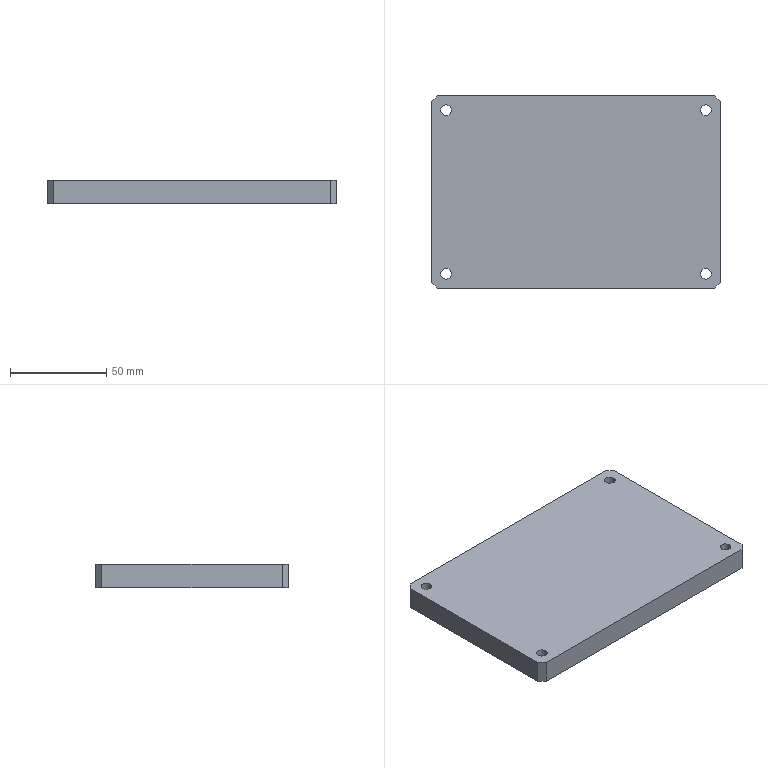Part | SolidWorks | features Chamfer 1, Extrusion 1, HoleWzd 1, ICE 1 | 1 solid | 95 faces | box 150 x 100 x 12 mm | volume 167862 mm3 | cylinder 48 | plane 47 | commonest cylinder face diameters 0.4 x32 5.5 x8 10 x8